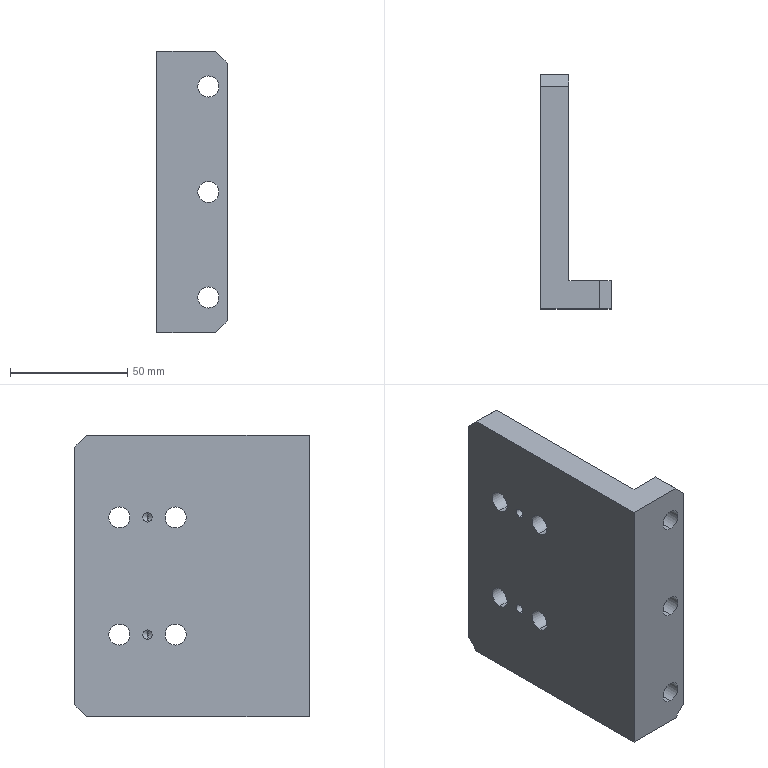Part | SolidWorks | features BaseBody 1 | 1 solid | 34 faces | box 30 x 100 x 120 mm | volume 163840 mm3 | cylinder 18 | plane 12 | cone 4 | commonest cylinder face diameters 9 x14 4 x4
STEP:
#1=CARTESIAN_POINT('',(5.,69.,-27.));
#2=VERTEX_POINT('',#1);
#3=CARTESIAN_POINT('',(5.,69.,-23.));
#4=VERTEX_POINT('',#3);
#5=CARTESIAN_POINT('',(5.,69.,-25.));
#6=DIRECTION('',(-1.,0.,0.));
#7=DIRECTION('',(0.,0.,1.));
#8=AXIS2_PLACEMENT_3D('',#5,#6,#7);
#9=CIRCLE('',#8,2.);
#10=EDGE_CURVE('',#2,#4,#9,.T.);
#11=ORIENTED_EDGE('',*,*,#10,.F.);
#12=CARTESIAN_POINT('',(0.,69.,-27.));
#13=VERTEX_POINT('',#12);
#14=CARTESIAN_POINT('',(0.,69.,-27.));
#15=DIRECTION('',(-1.,0.,0.));
#16=VECTOR('',#15,1000.);
#17=LINE('',#14,#16);
#18=EDGE_CURVE('',#2,#13,#17,.T.);
#19=ORIENTED_EDGE('',*,*,#18,.T.);
#20=CARTESIAN_POINT('',(0.,69.,-23.));
#21=VERTEX_POINT('',#20);
#22=CARTESIAN_POINT('',(0.,69.,-25.));
#23=DIRECTION('',(-1.,0.,0.));
#24=DIRECTION('',(0.,0.,1.));
#25=AXIS2_PLACEMENT_3D('',#22,#23,#24);
#26=CIRCLE('',#25,2.);
#27=EDGE_CURVE('',#13,#21,#26,.T.);
#28=ORIENTED_EDGE('',*,*,#27,.T.);
#29=CARTESIAN_POINT('',(0.,69.,-23.));
#30=DIRECTION('',(-1.,0.,0.));
#31=VECTOR('',#30,1000.);
#32=LINE('',#29,#31);
#33=EDGE_CURVE('',#4,#21,#32,.T.);
#34=ORIENTED_EDGE('',*,*,#33,.F.);
#35=EDGE_LOOP('',(#11,#19,#28,#34));
#36=FACE_OUTER_BOUND('',#35,.T.);
#37=CARTESIAN_POINT('',(0.,69.,-25.));
#38=DIRECTION('',(-1.,0.,0.));
#39=DIRECTION('',(0.,0.,1.));
#40=AXIS2_PLACEMENT_3D('',#37,#38,#39);
#41=CYLINDRICAL_SURFACE('',#40,2.);
#42=ADVANCED_FACE('',(#36),#41,.F.);
#43=CARTESIAN_POINT('',(6.202,69.,-25.));
#44=VERTEX_POINT('',#43);
#45=CARTESIAN_POINT('',(5.,69.,-23.));
#46=DIRECTION('',(-0.515,0.,0.8572));
#47=VECTOR('',#46,1000.);
#48=LINE('',#45,#47);
#49=EDGE_CURVE('',#44,#4,#48,.T.);
#50=ORIENTED_EDGE('',*,*,#49,.F.);
#51=CARTESIAN_POINT('',(5.,69.,-27.));
#52=DIRECTION('',(-0.515,0.,-0.8572));
#53=VECTOR('',#52,1000.);
#54=LINE('',#51,#53);
#55=EDGE_CURVE('',#44,#2,#54,.T.);
#56=ORIENTED_EDGE('',*,*,#55,.T.);
#57=ORIENTED_EDGE('',*,*,#10,.T.);
#58=EDGE_LOOP('',(#50,#56,#57));
#59=FACE_OUTER_BOUND('',#58,.T.);
#60=CARTESIAN_POINT('',(5.,69.,-25.));
#61=DIRECTION('',(-1.,0.,0.));
#62=DIRECTION('',(0.,0.,1.));
#63=AXIS2_PLACEMENT_3D('',#60,#61,#62);
#64=CONICAL_SURFACE('',#63,2.,1.03);
#65=ADVANCED_FACE('',(#59),#64,.F.);
#66=CARTESIAN_POINT('',(5.,69.,23.));
#67=VERTEX_POINT('',#66);
#68=CARTESIAN_POINT('',(5.,69.,27.));
#69=VERTEX_POINT('',#68);
#70=CARTESIAN_POINT('',(5.,69.,25.));
#71=DIRECTION('',(-1.,0.,0.));
#72=DIRECTION('',(0.,0.,1.));
#73=AXIS2_PLACEMENT_3D('',#70,#71,#72);
#74=CIRCLE('',#73,2.);
#75=EDGE_CURVE('',#67,#69,#74,.T.);
#76=ORIENTED_EDGE('',*,*,#75,.F.);
#77=CARTESIAN_POINT('',(0.,69.,23.));
#78=VERTEX_POINT('',#77);
#79=CARTESIAN_POINT('',(0.,69.,23.));
#80=DIRECTION('',(-1.,0.,0.));
#81=VECTOR('',#80,1000.);
#82=LINE('',#79,#81);
#83=EDGE_CURVE('',#67,#78,#82,.T.);
#84=ORIENTED_EDGE('',*,*,#83,.T.);
#85=CARTESIAN_POINT('',(0.,69.,27.));
#86=VERTEX_POINT('',#85);
#87=CARTESIAN_POINT('',(0.,69.,25.));
#88=DIRECTION('',(-1.,0.,0.));
#89=DIRECTION('',(0.,0.,1.));
#90=AXIS2_PLACEMENT_3D('',#87,#88,#89);
#91=CIRCLE('',#90,2.);
#92=EDGE_CURVE('',#78,#86,#91,.T.);
#93=ORIENTED_EDGE('',*,*,#92,.T.);
#94=CARTESIAN_POINT('',(0.,69.,27.));
#95=DIRECTION('',(-1.,0.,0.));
#96=VECTOR('',#95,1000.);
#97=LINE('',#94,#96);
#98=EDGE_CURVE('',#69,#86,#97,.T.);
#99=ORIENTED_EDGE('',*,*,#98,.F.);
#100=EDGE_LOOP('',(#76,#84,#93,#99));
#101=FACE_OUTER_BOUND('',#100,.T.);
#102=CARTESIAN_POINT('',(0.,69.,25.));
#103=DIRECTION('',(-1.,0.,0.));
#104=DIRECTION('',(0.,0.,1.));
#105=AXIS2_PLACEMENT_3D('',#102,#103,#104);
#106=CYLINDRICAL_SURFACE('',#105,2.);
#107=ADVANCED_FACE('',(#101),#106,.F.);
#108=CARTESIAN_POINT('',(6.202,69.,25.));
#109=VERTEX_POINT('',#108);
#110=CARTESIAN_POINT('',(5.,69.,27.));
#111=DIRECTION('',(-0.515,0.,0.8572));
#112=VECTOR('',#111,1000.);
#113=LINE('',#110,#112);
#114=EDGE_CURVE('',#109,#69,#113,.T.);
#115=ORIENTED_EDGE('',*,*,#114,.F.);
#116=CARTESIAN_POINT('',(5.,69.,23.));
#117=DIRECTION('',(-0.515,0.,-0.8572));
#118=VECTOR('',#117,1000.);
#119=LINE('',#116,#118);
#120=EDGE_CURVE('',#109,#67,#119,.T.);
#121=ORIENTED_EDGE('',*,*,#120,.T.);
#122=ORIENTED_EDGE('',*,*,#75,.T.);
#123=EDGE_LOOP('',(#115,#121,#122));
#124=FACE_OUTER_BOUND('',#123,.T.);
#125=CARTESIAN_POINT('',(5.,69.,25.));
#126=DIRECTION('',(-1.,0.,0.));
#127=DIRECTION('',(0.,0.,1.));
#128=AXIS2_PLACEMENT_3D('',#125,#126,#127);
#129=CONICAL_SURFACE('',#128,2.,1.03);
#130=ADVANCED_FACE('',(#124),#129,.F.);
#131=CARTESIAN_POINT('',(22.,0.,40.5));
#132=VERTEX_POINT('',#131);
#133=CARTESIAN_POINT('',(22.,0.,49.5));
#134=VERTEX_POINT('',#133);
#135=CARTESIAN_POINT('',(22.,0.,45.));
#136=DIRECTION('',(0.,1.,0.));
#137=DIRECTION('',(0.,0.,1.));
#138=AXIS2_PLACEMENT_3D('',#135,#136,#137);
#139=CIRCLE('',#138,4.5);
#140=EDGE_CURVE('',#132,#134,#139,.T.);
#141=ORIENTED_EDGE('',*,*,#140,.F.);
#142=CARTESIAN_POINT('',(22.,12.,40.5));
#143=VERTEX_POINT('',#142);
#144=CARTESIAN_POINT('',(22.,12.,40.5));
#145=DIRECTION('',(0.,1.,0.));
#146=VECTOR('',#145,1000.);
#147=LINE('',#144,#146);
#148=EDGE_CURVE('',#132,#143,#147,.T.);
#149=ORIENTED_EDGE('',*,*,#148,.T.);
#150=CARTESIAN_POINT('',(22.,12.,49.5));
#151=VERTEX_POINT('',#150);
#152=CARTESIAN_POINT('',(22.,12.,45.));
#153=DIRECTION('',(0.,1.,0.));
#154=DIRECTION('',(0.,0.,1.));
#155=AXIS2_PLACEMENT_3D('',#152,#153,#154);
#156=CIRCLE('',#155,4.5);
#157=EDGE_CURVE('',#143,#151,#156,.T.);
#158=ORIENTED_EDGE('',*,*,#157,.T.);
#159=CARTESIAN_POINT('',(22.,12.,49.5));
#160=DIRECTION('',(0.,1.,0.));
#161=VECTOR('',#160,1000.);
#162=LINE('',#159,#161);
#163=EDGE_CURVE('',#134,#151,#162,.T.);
#164=ORIENTED_EDGE('',*,*,#163,.F.);
#165=EDGE_LOOP('',(#141,#149,#158,#164));
#166=FACE_OUTER_BOUND('',#165,.T.);
#167=CARTESIAN_POINT('',(22.,12.,45.));
#168=DIRECTION('',(0.,1.,0.));
#169=DIRECTION('',(0.,0.,1.));
#170=AXIS2_PLACEMENT_3D('',#167,#168,#169);
#171=CYLINDRICAL_SURFACE('',#170,4.5);
#172=ADVANCED_FACE('',(#166),#171,.F.);
#173=CARTESIAN_POINT('',(22.,0.,-4.5));
#174=VERTEX_POINT('',#173);
#175=CARTESIAN_POINT('',(22.,0.,4.5));
#176=VERTEX_POINT('',#175);
#177=CARTESIAN_POINT('',(22.,0.,0.));
#178=DIRECTION('',(0.,1.,0.));
#179=DIRECTION('',(0.,0.,1.));
#180=AXIS2_PLACEMENT_3D('',#177,#178,#179);
#181=CIRCLE('',#180,4.5);
#182=EDGE_CURVE('',#174,#176,#181,.T.);
#183=ORIENTED_EDGE('',*,*,#182,.F.);
#184=CARTESIAN_POINT('',(22.,12.,-4.5));
#185=VERTEX_POINT('',#184);
#186=CARTESIAN_POINT('',(22.,12.,-4.5));
#187=DIRECTION('',(0.,1.,0.));
#188=VECTOR('',#187,1000.);
#189=LINE('',#186,#188);
#190=EDGE_CURVE('',#174,#185,#189,.T.);
#191=ORIENTED_EDGE('',*,*,#190,.T.);
#192=CARTESIAN_POINT('',(22.,12.,4.5));
#193=VERTEX_POINT('',#192);
#194=CARTESIAN_POINT('',(22.,12.,0.));
#195=DIRECTION('',(0.,1.,0.));
#196=DIRECTION('',(0.,0.,1.));
#197=AXIS2_PLACEMENT_3D('',#194,#195,#196);
#198=CIRCLE('',#197,4.5);
#199=EDGE_CURVE('',#185,#193,#198,.T.);
#200=ORIENTED_EDGE('',*,*,#199,.T.);
#201=CARTESIAN_POINT('',(22.,12.,4.5));
#202=DIRECTION('',(0.,1.,0.));
#203=VECTOR('',#202,1000.);
#204=LINE('',#201,#203);
#205=EDGE_CURVE('',#176,#193,#204,.T.);
#206=ORIENTED_EDGE('',*,*,#205,.F.);
#207=EDGE_LOOP('',(#183,#191,#200,#206));
#208=FACE_OUTER_BOUND('',#207,.T.);
#209=CARTESIAN_POINT('',(22.,12.,0.));
#210=DIRECTION('',(0.,1.,0.));
#211=DIRECTION('',(0.,0.,1.));
#212=AXIS2_PLACEMENT_3D('',#209,#210,#211);
#213=CYLINDRICAL_SURFACE('',#212,4.5);
#214=ADVANCED_FACE('',(#208),#213,.F.);
#215=CARTESIAN_POINT('',(22.,0.,-49.5));
#216=VERTEX_POINT('',#215);
#217=CARTESIAN_POINT('',(22.,0.,-40.5));
#218=VERTEX_POINT('',#217);
#219=CARTESIAN_POINT('',(22.,0.,-45.));
#220=DIRECTION('',(0.,1.,0.));
#221=DIRECTION('',(0.,0.,1.));
#222=AXIS2_PLACEMENT_3D('',#219,#220,#221);
#223=CIRCLE('',#222,4.5);
#224=EDGE_CURVE('',#216,#218,#223,.T.);
#225=ORIENTED_EDGE('',*,*,#224,.F.);
#226=CARTESIAN_POINT('',(22.,12.,-49.5));
#227=VERTEX_POINT('',#226);
#228=CARTESIAN_POINT('',(22.,12.,-49.5));
#229=DIRECTION('',(0.,1.,0.));
#230=VECTOR('',#229,1000.);
#231=LINE('',#228,#230);
#232=EDGE_CURVE('',#216,#227,#231,.T.);
#233=ORIENTED_EDGE('',*,*,#232,.T.);
#234=CARTESIAN_POINT('',(22.,12.,-40.5));
#235=VERTEX_POINT('',#234);
#236=CARTESIAN_POINT('',(22.,12.,-45.));
#237=DIRECTION('',(0.,1.,0.));
#238=DIRECTION('',(0.,0.,1.));
#239=AXIS2_PLACEMENT_3D('',#236,#237,#238);
#240=CIRCLE('',#239,4.5);
#241=EDGE_CURVE('',#227,#235,#240,.T.);
#242=ORIENTED_EDGE('',*,*,#241,.T.);
#243=CARTESIAN_POINT('',(22.,12.,-40.5));
#244=DIRECTION('',(0.,1.,0.));
#245=VECTOR('',#244,1000.);
#246=LINE('',#243,#245);
#247=EDGE_CURVE('',#218,#235,#246,.T.);
#248=ORIENTED_EDGE('',*,*,#247,.F.);
#249=EDGE_LOOP('',(#225,#233,#242,#248));
#250=FACE_OUTER_BOUND('',#249,.T.);
#251=CARTESIAN_POINT('',(22.,12.,-45.));
#252=DIRECTION('',(0.,1.,0.));
#253=DIRECTION('',(0.,0.,1.));
#254=AXIS2_PLACEMENT_3D('',#251,#252,#253);
#255=CYLINDRICAL_SURFACE('',#254,4.5);
#256=ADVANCED_FACE('',(#250),#255,.F.);
#257=CARTESIAN_POINT('',(0.,81.,29.5));
#258=VERTEX_POINT('',#257);
#259=CARTESIAN_POINT('',(0.,81.,20.5));
#260=VERTEX_POINT('',#259);
#261=CARTESIAN_POINT('',(0.,81.,25.));
#262=DIRECTION('',(1.,0.,0.));
#263=DIRECTION('',(0.,0.,-1.));
#264=AXIS2_PLACEMENT_3D('',#261,#262,#263);
#265=CIRCLE('',#264,4.5);
#266=EDGE_CURVE('',#258,#260,#265,.T.);
#267=ORIENTED_EDGE('',*,*,#266,.F.);
#268=CARTESIAN_POINT('',(12.,81.,29.5));
#269=VERTEX_POINT('',#268);
#270=CARTESIAN_POINT('',(12.,81.,29.5));
#271=DIRECTION('',(1.,0.,0.));
#272=VECTOR('',#271,1000.);
#273=LINE('',#270,#272);
#274=EDGE_CURVE('',#258,#269,#273,.T.);
#275=ORIENTED_EDGE('',*,*,#274,.T.);
#276=CARTESIAN_POINT('',(12.,81.,20.5));
#277=VERTEX_POINT('',#276);
#278=CARTESIAN_POINT('',(12.,81.,25.));
#279=DIRECTION('',(1.,0.,0.));
#280=DIRECTION('',(0.,0.,-1.));
#281=AXIS2_PLACEMENT_3D('',#278,#279,#280);
#282=CIRCLE('',#281,4.5);
#283=EDGE_CURVE('',#269,#277,#282,.T.);
#284=ORIENTED_EDGE('',*,*,#283,.T.);
#285=CARTESIAN_POINT('',(12.,81.,20.5));
#286=DIRECTION('',(1.,0.,0.));
#287=VECTOR('',#286,1000.);
#288=LINE('',#285,#287);
#289=EDGE_CURVE('',#260,#277,#288,.T.);
#290=ORIENTED_EDGE('',*,*,#289,.F.);
#291=EDGE_LOOP('',(#267,#275,#284,#290));
#292=FACE_OUTER_BOUND('',#291,.T.);
#293=CARTESIAN_POINT('',(12.,81.,25.));
#294=DIRECTION('',(1.,0.,0.));
#295=DIRECTION('',(0.,0.,-1.));
#296=AXIS2_PLACEMENT_3D('',#293,#294,#295);
#297=CYLINDRICAL_SURFACE('',#296,4.5);
#298=ADVANCED_FACE('',(#292),#297,.F.);
#299=CARTESIAN_POINT('',(0.,57.,-20.5));
#300=VERTEX_POINT('',#299);
#301=CARTESIAN_POINT('',(0.,57.,-29.5));
#302=VERTEX_POINT('',#301);
#303=CARTESIAN_POINT('',(0.,57.,-25.));
#304=DIRECTION('',(1.,0.,0.));
#305=DIRECTION('',(0.,0.,-1.));
#306=AXIS2_PLACEMENT_3D('',#303,#304,#305);
#307=CIRCLE('',#306,4.5);
#308=EDGE_CURVE('',#300,#302,#307,.T.);
#309=ORIENTED_EDGE('',*,*,#308,.F.);
#310=CARTESIAN_POINT('',(12.,57.,-20.5));
#311=VERTEX_POINT('',#310);
#312=CARTESIAN_POINT('',(12.,57.,-20.5));
#313=DIRECTION('',(1.,0.,0.));
#314=VECTOR('',#313,1000.);
#315=LINE('',#312,#314);
#316=EDGE_CURVE('',#300,#311,#315,.T.);
#317=ORIENTED_EDGE('',*,*,#316,.T.);
#318=CARTESIAN_POINT('',(12.,57.,-29.5));
#319=VERTEX_POINT('',#318);
#320=CARTESIAN_POINT('',(12.,57.,-25.));
#321=DIRECTION('',(1.,0.,0.));
#322=DIRECTION('',(0.,0.,-1.));
#323=AXIS2_PLACEMENT_3D('',#320,#321,#322);
#324=CIRCLE('',#323,4.5);
#325=EDGE_CURVE('',#311,#319,#324,.T.);
#326=ORIENTED_EDGE('',*,*,#325,.T.);
#327=CARTESIAN_POINT('',(12.,57.,-29.5));
#328=DIRECTION('',(1.,0.,0.));
#329=VECTOR('',#328,1000.);
#330=LINE('',#327,#329);
#331=EDGE_CURVE('',#302,#319,#330,.T.);
#332=ORIENTED_EDGE('',*,*,#331,.F.);
#333=EDGE_LOOP('',(#309,#317,#326,#332));
#334=FACE_OUTER_BOUND('',#333,.T.);
#335=CARTESIAN_POINT('',(12.,57.,-25.));
#336=DIRECTION('',(1.,0.,0.));
#337=DIRECTION('',(0.,0.,-1.));
#338=AXIS2_PLACEMENT_3D('',#335,#336,#337);
#339=CYLINDRICAL_SURFACE('',#338,4.5);
#340=ADVANCED_FACE('',(#334),#339,.F.);
#341=CARTESIAN_POINT('',(0.,57.,29.5));
#342=VERTEX_POINT('',#341);
#343=CARTESIAN_POINT('',(0.,57.,20.5));
#344=VERTEX_POINT('',#343);
#345=CARTESIAN_POINT('',(0.,57.,25.));
#346=DIRECTION('',(1.,0.,0.));
#347=DIRECTION('',(0.,0.,-1.));
#348=AXIS2_PLACEMENT_3D('',#345,#346,#347);
#349=CIRCLE('',#348,4.5);
#350=EDGE_CURVE('',#342,#344,#349,.T.);
#351=ORIENTED_EDGE('',*,*,#350,.F.);
#352=CARTESIAN_POINT('',(12.,57.,29.5));
#353=VERTEX_POINT('',#352);
#354=CARTESIAN_POINT('',(12.,57.,29.5));
#355=DIRECTION('',(1.,0.,0.));
#356=VECTOR('',#355,1000.);
#357=LINE('',#354,#356);
#358=EDGE_CURVE('',#342,#353,#357,.T.);
#359=ORIENTED_EDGE('',*,*,#358,.T.);
#360=CARTESIAN_POINT('',(12.,57.,20.5));
#361=VERTEX_POINT('',#360);
#362=CARTESIAN_POINT('',(12.,57.,25.));
#363=DIRECTION('',(1.,0.,0.));
#364=DIRECTION('',(0.,0.,-1.));
#365=AXIS2_PLACEMENT_3D('',#362,#363,#364);
#366=CIRCLE('',#365,4.5);
#367=EDGE_CURVE('',#353,#361,#366,.T.);
#368=ORIENTED_EDGE('',*,*,#367,.T.);
#369=CARTESIAN_POINT('',(12.,57.,20.5));
#370=DIRECTION('',(1.,0.,0.));
#371=VECTOR('',#370,1000.);
#372=LINE('',#369,#371);
#373=EDGE_CURVE('',#344,#361,#372,.T.);
#374=ORIENTED_EDGE('',*,*,#373,.F.);
#375=EDGE_LOOP('',(#351,#359,#368,#374));
#376=FACE_OUTER_BOUND('',#375,.T.);
#377=CARTESIAN_POINT('',(12.,57.,25.));
#378=DIRECTION('',(1.,0.,0.));
#379=DIRECTION('',(0.,0.,-1.));
#380=AXIS2_PLACEMENT_3D('',#377,#378,#379);
#381=CYLINDRICAL_SURFACE('',#380,4.5);
#382=ADVANCED_FACE('',(#376),#381,.F.);
#383=CARTESIAN_POINT('',(0.,81.,-20.5));
#384=VERTEX_POINT('',#383);
#385=CARTESIAN_POINT('',(0.,81.,-29.5));
#386=VERTEX_POINT('',#385);
#387=CARTESIAN_POINT('',(0.,81.,-25.));
#388=DIRECTION('',(1.,0.,0.));
#389=DIRECTION('',(0.,0.,-1.));
#390=AXIS2_PLACEMENT_3D('',#387,#388,#389);
#391=CIRCLE('',#390,4.5);
#392=EDGE_CURVE('',#384,#386,#391,.T.);
#393=ORIENTED_EDGE('',*,*,#392,.F.);
#394=CARTESIAN_POINT('',(12.,81.,-20.5));
#395=VERTEX_POINT('',#394);
#396=CARTESIAN_POINT('',(12.,81.,-20.5));
#397=DIRECTION('',(1.,0.,0.));
#398=VECTOR('',#397,1000.);
#399=LINE('',#396,#398);
#400=EDGE_CURVE('',#384,#395,#399,.T.);
#401=ORIENTED_EDGE('',*,*,#400,.T.);
#402=CARTESIAN_POINT('',(12.,81.,-29.5));
#403=VERTEX_POINT('',#402);
#404=CARTESIAN_POINT('',(12.,81.,-25.));
#405=DIRECTION('',(1.,0.,0.));
#406=DIRECTION('',(0.,0.,-1.));
#407=AXIS2_PLACEMENT_3D('',#404,#405,#406);
#408=CIRCLE('',#407,4.5);
#409=EDGE_CURVE('',#395,#403,#408,.T.);
#410=ORIENTED_EDGE('',*,*,#409,.T.);
#411=CARTESIAN_POINT('',(12.,81.,-29.5));
#412=DIRECTION('',(1.,0.,0.));
#413=VECTOR('',#412,1000.);
#414=LINE('',#411,#413);
#415=EDGE_CURVE('',#386,#403,#414,.T.);
#416=ORIENTED_EDGE('',*,*,#415,.F.);
#417=EDGE_LOOP('',(#393,#401,#410,#416));
#418=FACE_OUTER_BOUND('',#417,.T.);
#419=CARTESIAN_POINT('',(12.,81.,-25.));
#420=DIRECTION('',(1.,0.,0.));
#421=DIRECTION('',(0.,0.,-1.));
#422=AXIS2_PLACEMENT_3D('',#419,#420,#421);
#423=CYLINDRICAL_SURFACE('',#422,4.5);
#424=ADVANCED_FACE('',(#418),#423,.F.);
#425=CARTESIAN_POINT('',(0.,95.,60.));
#426=VERTEX_POINT('',#425);
#427=CARTESIAN_POINT('',(0.,100.,55.));
#428=VERTEX_POINT('',#427);
#429=CARTESIAN_POINT('',(0.,100.,55.));
#430=DIRECTION('',(0.,0.7071,-0.7071));
#431=VECTOR('',#430,1000.);
#432=LINE('',#429,#431);
#433=EDGE_CURVE('',#426,#428,#432,.T.);
#434=ORIENTED_EDGE('',*,*,#433,.F.);
#435=CARTESIAN_POINT('',(12.,95.,60.));
#436=VERTEX_POINT('',#435);
#437=CARTESIAN_POINT('',(0.,95.,60.));
#438=DIRECTION('',(-1.,0.,0.));
#439=VECTOR('',#438,1000.);
#440=LINE('',#437,#439);
#441=EDGE_CURVE('',#436,#426,#440,.T.);
#442=ORIENTED_EDGE('',*,*,#441,.F.);
#443=CARTESIAN_POINT('',(12.,100.,55.));
#444=VERTEX_POINT('',#443);
#445=CARTESIAN_POINT('',(12.,97.5,57.5));
#446=DIRECTION('',(0.,-0.7071,0.7071));
#447=VECTOR('',#446,1000.);
#448=LINE('',#445,#447);
#449=EDGE_CURVE('',#444,#436,#448,.T.);
#450=ORIENTED_EDGE('',*,*,#449,.F.);
#451=CARTESIAN_POINT('',(12.,100.,55.));
#452=DIRECTION('',(1.,0.,0.));
#453=VECTOR('',#452,1000.);
#454=LINE('',#451,#453);
#455=EDGE_CURVE('',#428,#444,#454,.T.);
#456=ORIENTED_EDGE('',*,*,#455,.F.);
#457=EDGE_LOOP('',(#434,#442,#450,#456));
#458=FACE_OUTER_BOUND('',#457,.T.);
#459=CARTESIAN_POINT('',(0.,100.,55.));
#460=DIRECTION('',(0.,0.7071,0.7071));
#461=DIRECTION('',(1.,0.,0.));
#462=AXIS2_PLACEMENT_3D('',#459,#460,#461);
#463=PLANE('',#462);
#464=ADVANCED_FACE('',(#458),#463,.T.);
#465=CARTESIAN_POINT('',(0.,100.,-55.));
#466=VERTEX_POINT('',#465);
#467=CARTESIAN_POINT('',(0.,95.,-60.));
#468=VERTEX_POINT('',#467);
#469=CARTESIAN_POINT('',(0.,95.,-60.));
#470=DIRECTION('',(0.,-0.7071,-0.7071));
#471=VECTOR('',#470,1000.);
#472=LINE('',#469,#471);
#473=EDGE_CURVE('',#466,#468,#472,.T.);
#474=ORIENTED_EDGE('',*,*,#473,.F.);
#475=CARTESIAN_POINT('',(12.,100.,-55.));
#476=VERTEX_POINT('',#475);
#477=CARTESIAN_POINT('',(0.,100.,-55.));
#478=DIRECTION('',(-1.,0.,0.));
#479=VECTOR('',#478,1000.);
#480=LINE('',#477,#479);
#481=EDGE_CURVE('',#476,#466,#480,.T.);
#482=ORIENTED_EDGE('',*,*,#481,.F.);
#483=CARTESIAN_POINT('',(12.,95.,-60.));
#484=VERTEX_POINT('',#483);
#485=CARTESIAN_POINT('',(12.,157.5,2.5));
#486=DIRECTION('',(0.,0.7071,0.7071));
#487=VECTOR('',#486,1000.);
#488=LINE('',#485,#487);
#489=EDGE_CURVE('',#484,#476,#488,.T.);
#490=ORIENTED_EDGE('',*,*,#489,.F.);
#491=CARTESIAN_POINT('',(0.,95.,-60.));
#492=DIRECTION('',(1.,0.,0.));
#493=VECTOR('',#492,1000.);
#494=LINE('',#491,#493);
#495=EDGE_CURVE('',#468,#484,#494,.T.);
#496=ORIENTED_EDGE('',*,*,#495,.F.);
#497=EDGE_LOOP('',(#474,#482,#490,#496));
#498=FACE_OUTER_BOUND('',#497,.T.);
#499=CARTESIAN_POINT('',(0.,95.,-60.));
#500=DIRECTION('',(0.,-0.7071,0.7071));
#501=DIRECTION('',(-1.,0.,0.));
#502=AXIS2_PLACEMENT_3D('',#499,#500,#501);
#503=PLANE('',#502);
#504=ADVANCED_FACE('',(#498),#503,.F.);
#505=CARTESIAN_POINT('',(30.,12.,-55.));
#506=VERTEX_POINT('',#505);
#507=CARTESIAN_POINT('',(25.,12.,-60.));
#508=VERTEX_POINT('',#507);
#509=CARTESIAN_POINT('',(72.5,12.,-12.5));
#510=DIRECTION('',(-0.7071,0.,-0.7071));
#511=VECTOR('',#510,1000.);
#512=LINE('',#509,#511);
#513=EDGE_CURVE('',#506,#508,#512,.T.);
#514=ORIENTED_EDGE('',*,*,#513,.F.);
#515=CARTESIAN_POINT('',(30.,0.,-55.));
#516=VERTEX_POINT('',#515);
#517=CARTESIAN_POINT('',(30.,12.,-55.));
#518=DIRECTION('',(0.,1.,0.));
#519=VECTOR('',#518,1000.);
#520=LINE('',#517,#519);
#521=EDGE_CURVE('',#516,#506,#520,.T.);
#522=ORIENTED_EDGE('',*,*,#521,.F.);
#523=CARTESIAN_POINT('',(25.,0.,-60.));
#524=VERTEX_POINT('',#523);
#525=CARTESIAN_POINT('',(25.,0.,-60.));
#526=DIRECTION('',(0.7071,0.,0.7071));
#527=VECTOR('',#526,1000.);
#528=LINE('',#525,#527);
#529=EDGE_CURVE('',#524,#516,#528,.T.);
#530=ORIENTED_EDGE('',*,*,#529,.F.);
#531=CARTESIAN_POINT('',(25.,0.,-60.));
#532=DIRECTION('',(0.,-1.,0.));
#533=VECTOR('',#532,1000.);
#534=LINE('',#531,#533);
#535=EDGE_CURVE('',#508,#524,#534,.T.);
#536=ORIENTED_EDGE('',*,*,#535,.F.);
#537=EDGE_LOOP('',(#514,#522,#530,#536));
#538=FACE_OUTER_BOUND('',#537,.T.);
#539=CARTESIAN_POINT('',(25.,0.,-60.));
#540=DIRECTION('',(-0.7071,0.,0.7071));
#541=DIRECTION('',(0.,1.,0.));
#542=AXIS2_PLACEMENT_3D('',#539,#540,#541);
#543=PLANE('',#542);
#544=ADVANCED_FACE('',(#538),#543,.F.);
#545=CARTESIAN_POINT('',(25.,12.,60.));
#546=VERTEX_POINT('',#545);
#547=CARTESIAN_POINT('',(30.,12.,55.));
#548=VERTEX_POINT('',#547);
#549=CARTESIAN_POINT('',(12.5,12.,72.5));
#550=DIRECTION('',(0.7071,0.,-0.7071));
#551=VECTOR('',#550,1000.);
#552=LINE('',#549,#551);
#553=EDGE_CURVE('',#546,#548,#552,.T.);
#554=ORIENTED_EDGE('',*,*,#553,.F.);
#555=CARTESIAN_POINT('',(25.,0.,60.));
#556=VERTEX_POINT('',#555);
#557=CARTESIAN_POINT('',(25.,12.,60.));
#558=DIRECTION('',(0.,1.,0.));
#559=VECTOR('',#558,1000.);
#560=LINE('',#557,#559);
#561=EDGE_CURVE('',#556,#546,#560,.T.);
#562=ORIENTED_EDGE('',*,*,#561,.F.);
#563=CARTESIAN_POINT('',(30.,0.,55.));
#564=VERTEX_POINT('',#563);
#565=CARTESIAN_POINT('',(30.,0.,55.));
#566=DIRECTION('',(-0.7071,0.,0.7071));
#567=VECTOR('',#566,1000.);
#568=LINE('',#565,#567);
#569=EDGE_CURVE('',#564,#556,#568,.T.);
#570=ORIENTED_EDGE('',*,*,#569,.F.);
#571=CARTESIAN_POINT('',(30.,0.,55.));
#572=DIRECTION('',(0.,-1.,0.));
#573=VECTOR('',#572,1000.);
#574=LINE('',#571,#573);
#575=EDGE_CURVE('',#548,#564,#574,.T.);
#576=ORIENTED_EDGE('',*,*,#575,.F.);
#577=EDGE_LOOP('',(#554,#562,#570,#576));
#578=FACE_OUTER_BOUND('',#577,.T.);
#579=CARTESIAN_POINT('',(30.,12.,55.));
#580=DIRECTION('',(0.7071,0.,0.7071));
#581=DIRECTION('',(0.,-1.,0.));
#582=AXIS2_PLACEMENT_3D('',#579,#580,#581);
#583=PLANE('',#582);
#584=ADVANCED_FACE('',(#578),#583,.T.);
#585=CARTESIAN_POINT('',(12.,12.,-60.));
#586=VERTEX_POINT('',#585);
#587=CARTESIAN_POINT('',(0.,12.,-60.));
#588=DIRECTION('',(1.,0.,0.));
#589=VECTOR('',#588,1000.);
#590=LINE('',#587,#589);
#591=EDGE_CURVE('',#586,#508,#590,.T.);
#592=ORIENTED_EDGE('',*,*,#591,.T.);
#593=ORIENTED_EDGE('',*,*,#535,.T.);
#594=CARTESIAN_POINT('',(0.,0.,-60.));
#595=VERTEX_POINT('',#594);
#596=CARTESIAN_POINT('',(0.,0.,-60.));
#597=DIRECTION('',(1.,0.,0.));
#598=VECTOR('',#597,1000.);
#599=LINE('',#596,#598);
#600=EDGE_CURVE('',#595,#524,#599,.T.);
#601=ORIENTED_EDGE('',*,*,#600,.F.);
#602=CARTESIAN_POINT('',(0.,100.,-60.));
#603=DIRECTION('',(0.,-1.,0.));
#604=VECTOR('',#603,1000.);
#605=LINE('',#602,#604);
#606=EDGE_CURVE('',#468,#595,#605,.T.);
#607=ORIENTED_EDGE('',*,*,#606,.F.);
#608=ORIENTED_EDGE('',*,*,#495,.T.);
#609=CARTESIAN_POINT('',(12.,100.,-60.));
#610=DIRECTION('',(0.,-1.,0.));
#611=VECTOR('',#610,1000.);
#612=LINE('',#609,#611);
#613=EDGE_CURVE('',#484,#586,#612,.T.);
#614=ORIENTED_EDGE('',*,*,#613,.T.);
#615=EDGE_LOOP('',(#592,#593,#601,#607,#608,#614));
#616=FACE_OUTER_BOUND('',#615,.T.);
#617=CARTESIAN_POINT('',(0.,0.,-60.));
#618=DIRECTION('',(0.,0.,-1.));
#619=DIRECTION('',(0.,-1.,0.));
#620=AXIS2_PLACEMENT_3D('',#617,#618,#619);
#621=PLANE('',#620);
#622=ADVANCED_FACE('',(#616),#621,.T.);
#623=CARTESIAN_POINT('',(0.,0.,60.));
#624=VERTEX_POINT('',#623);
#625=CARTESIAN_POINT('',(0.,0.,60.));
#626=DIRECTION('',(1.,0.,0.));
#627=VECTOR('',#626,1000.);
#628=LINE('',#625,#627);
#629=EDGE_CURVE('',#624,#556,#628,.T.);
#630=ORIENTED_EDGE('',*,*,#629,.T.);
#631=ORIENTED_EDGE('',*,*,#561,.T.);
#632=CARTESIAN_POINT('',(12.,12.,60.));
#633=VERTEX_POINT('',#632);
#634=CARTESIAN_POINT('',(0.,12.,60.));
#635=DIRECTION('',(1.,0.,0.));
#636=VECTOR('',#635,1000.);
#637=LINE('',#634,#636);
#638=EDGE_CURVE('',#633,#546,#637,.T.);
#639=ORIENTED_EDGE('',*,*,#638,.F.);
#640=CARTESIAN_POINT('',(12.,100.,60.));
#641=DIRECTION('',(0.,-1.,0.));
#642=VECTOR('',#641,1000.);
#643=LINE('',#640,#642);
#644=EDGE_CURVE('',#436,#633,#643,.T.);
#645=ORIENTED_EDGE('',*,*,#644,.F.);
#646=ORIENTED_EDGE('',*,*,#441,.T.);
#647=CARTESIAN_POINT('',(0.,100.,60.));
#648=DIRECTION('',(0.,-1.,0.));
#649=VECTOR('',#648,1000.);
#650=LINE('',#647,#649);
#651=EDGE_CURVE('',#426,#624,#650,.T.);
#652=ORIENTED_EDGE('',*,*,#651,.T.);
#653=EDGE_LOOP('',(#630,#631,#639,#645,#646,#652));
#654=FACE_OUTER_BOUND('',#653,.T.);
#655=CARTESIAN_POINT('',(0.,0.,60.));
#656=DIRECTION('',(0.,0.,-1.));
#657=DIRECTION('',(0.,-1.,0.));
#658=AXIS2_PLACEMENT_3D('',#655,#656,#657);
#659=PLANE('',#658);
#660=ADVANCED_FACE('',(#654),#659,.F.);
#661=CARTESIAN_POINT('',(0.,81.,-25.));
#662=DIRECTION('',(1.,0.,0.));
#663=DIRECTION('',(0.,0.,-1.));
#664=AXIS2_PLACEMENT_3D('',#661,#662,#663);
#665=CIRCLE('',#664,4.5);
#666=EDGE_CURVE('',#386,#384,#665,.T.);
#667=ORIENTED_EDGE('',*,*,#666,.T.);
#668=ORIENTED_EDGE('',*,*,#392,.T.);
#669=EDGE_LOOP('',(#667,#668));
#670=FACE_BOUND('',#669,.T.);
#671=CARTESIAN_POINT('',(0.,57.,25.));
#672=DIRECTION('',(1.,0.,0.));
#673=DIRECTION('',(0.,0.,-1.));
#674=AXIS2_PLACEMENT_3D('',#671,#672,#673);
#675=CIRCLE('',#674,4.5);
#676=EDGE_CURVE('',#344,#342,#675,.T.);
#677=ORIENTED_EDGE('',*,*,#676,.T.);
#678=ORIENTED_EDGE('',*,*,#350,.T.);
#679=EDGE_LOOP('',(#677,#678));
#680=FACE_BOUND('',#679,.T.);
#681=CARTESIAN_POINT('',(0.,57.,-25.));
#682=DIRECTION('',(1.,0.,0.));
#683=DIRECTION('',(0.,0.,-1.));
#684=AXIS2_PLACEMENT_3D('',#681,#682,#683);
#685=CIRCLE('',#684,4.5);
#686=EDGE_CURVE('',#302,#300,#685,.T.);
#687=ORIENTED_EDGE('',*,*,#686,.T.);
#688=ORIENTED_EDGE('',*,*,#308,.T.);
#689=EDGE_LOOP('',(#687,#688));
#690=FACE_BOUND('',#689,.T.);
#691=CARTESIAN_POINT('',(0.,81.,25.));
#692=DIRECTION('',(1.,0.,0.));
#693=DIRECTION('',(0.,0.,-1.));
#694=AXIS2_PLACEMENT_3D('',#691,#692,#693);
#695=CIRCLE('',#694,4.5);
#696=EDGE_CURVE('',#260,#258,#695,.T.);
#697=ORIENTED_EDGE('',*,*,#696,.T.);
#698=ORIENTED_EDGE('',*,*,#266,.T.);
#699=EDGE_LOOP('',(#697,#698));
#700=FACE_BOUND('',#699,.T.);
#701=CARTESIAN_POINT('',(0.,69.,25.));
#702=DIRECTION('',(-1.,0.,0.));
#703=DIRECTION('',(0.,0.,1.));
#704=AXIS2_PLACEMENT_3D('',#701,#702,#703);
#705=CIRCLE('',#704,2.);
#706=EDGE_CURVE('',#86,#78,#705,.T.);
#707=ORIENTED_EDGE('',*,*,#706,.F.);
#708=ORIENTED_EDGE('',*,*,#92,.F.);
#709=EDGE_LOOP('',(#707,#708));
#710=FACE_BOUND('',#709,.T.);
#711=CARTESIAN_POINT('',(0.,69.,-25.));
#712=DIRECTION('',(-1.,0.,0.));
#713=DIRECTION('',(0.,0.,1.));
#714=AXIS2_PLACEMENT_3D('',#711,#712,#713);
#715=CIRCLE('',#714,2.);
#716=EDGE_CURVE('',#21,#13,#715,.T.);
#717=ORIENTED_EDGE('',*,*,#716,.F.);
#718=ORIENTED_EDGE('',*,*,#27,.F.);
#719=EDGE_LOOP('',(#717,#718));
#720=FACE_BOUND('',#719,.T.);
#721=CARTESIAN_POINT('',(0.,100.,60.));
#722=DIRECTION('',(0.,0.,-1.));
#723=VECTOR('',#722,1000.);
#724=LINE('',#721,#723);
#725=EDGE_CURVE('',#428,#466,#724,.T.);
#726=ORIENTED_EDGE('',*,*,#725,.T.);
#727=ORIENTED_EDGE('',*,*,#473,.T.);
#728=ORIENTED_EDGE('',*,*,#606,.T.);
#729=CARTESIAN_POINT('',(0.,0.,60.));
#730=DIRECTION('',(0.,0.,-1.));
#731=VECTOR('',#730,1000.);
#732=LINE('',#729,#731);
#733=EDGE_CURVE('',#624,#595,#732,.T.);
#734=ORIENTED_EDGE('',*,*,#733,.F.);
#735=ORIENTED_EDGE('',*,*,#651,.F.);
#736=ORIENTED_EDGE('',*,*,#433,.T.);
#737=EDGE_LOOP('',(#726,#727,#728,#734,#735,#736));
#738=FACE_OUTER_BOUND('',#737,.T.);
#739=CARTESIAN_POINT('',(0.,100.,60.));
#740=DIRECTION('',(1.,0.,0.));
#741=DIRECTION('',(0.,1.,0.));
#742=AXIS2_PLACEMENT_3D('',#739,#740,#741);
#743=PLANE('',#742);
#744=ADVANCED_FACE('',(#670,#680,#690,#700,#710,#720,#738),#743,.F.);
#745=CARTESIAN_POINT('',(12.,100.,60.));
#746=DIRECTION('',(0.,0.,-1.));
#747=VECTOR('',#746,1000.);
#748=LINE('',#745,#747);
#749=EDGE_CURVE('',#444,#476,#748,.T.);
#750=ORIENTED_EDGE('',*,*,#749,.T.);
#751=ORIENTED_EDGE('',*,*,#481,.T.);
#752=ORIENTED_EDGE('',*,*,#725,.F.);
#753=ORIENTED_EDGE('',*,*,#455,.T.);
#754=EDGE_LOOP('',(#750,#751,#752,#753));
#755=FACE_OUTER_BOUND('',#754,.T.);
#756=CARTESIAN_POINT('',(0.,100.,60.));
#757=DIRECTION('',(0.,1.,0.));
#758=DIRECTION('',(1.,0.,0.));
#759=AXIS2_PLACEMENT_3D('',#756,#757,#758);
#760=PLANE('',#759);
#761=ADVANCED_FACE('',(#755),#760,.T.);
#762=CARTESIAN_POINT('',(12.,81.,-25.));
#763=DIRECTION('',(1.,0.,0.));
#764=DIRECTION('',(0.,0.,-1.));
#765=AXIS2_PLACEMENT_3D('',#762,#763,#764);
#766=CIRCLE('',#765,4.5);
#767=EDGE_CURVE('',#403,#395,#766,.T.);
#768=ORIENTED_EDGE('',*,*,#767,.F.);
#769=ORIENTED_EDGE('',*,*,#409,.F.);
#770=EDGE_LOOP('',(#768,#769));
#771=FACE_BOUND('',#770,.T.);
#772=CARTESIAN_POINT('',(12.,57.,25.));
#773=DIRECTION('',(1.,0.,0.));
#774=DIRECTION('',(0.,0.,-1.));
#775=AXIS2_PLACEMENT_3D('',#772,#773,#774);
#776=CIRCLE('',#775,4.5);
#777=EDGE_CURVE('',#361,#353,#776,.T.);
#778=ORIENTED_EDGE('',*,*,#777,.F.);
#779=ORIENTED_EDGE('',*,*,#367,.F.);
#780=EDGE_LOOP('',(#778,#779));
#781=FACE_BOUND('',#780,.T.);
#782=CARTESIAN_POINT('',(12.,57.,-25.));
#783=DIRECTION('',(1.,0.,0.));
#784=DIRECTION('',(0.,0.,-1.));
#785=AXIS2_PLACEMENT_3D('',#782,#783,#784);
#786=CIRCLE('',#785,4.5);
#787=EDGE_CURVE('',#319,#311,#786,.T.);
#788=ORIENTED_EDGE('',*,*,#787,.F.);
#789=ORIENTED_EDGE('',*,*,#325,.F.);
#790=EDGE_LOOP('',(#788,#789));
#791=FACE_BOUND('',#790,.T.);
#792=CARTESIAN_POINT('',(12.,81.,25.));
#793=DIRECTION('',(1.,0.,0.));
#794=DIRECTION('',(0.,0.,-1.));
#795=AXIS2_PLACEMENT_3D('',#792,#793,#794);
#796=CIRCLE('',#795,4.5);
#797=EDGE_CURVE('',#277,#269,#796,.T.);
#798=ORIENTED_EDGE('',*,*,#797,.F.);
#799=ORIENTED_EDGE('',*,*,#283,.F.);
#800=EDGE_LOOP('',(#798,#799));
#801=FACE_BOUND('',#800,.T.);
#802=ORIENTED_EDGE('',*,*,#613,.F.);
#803=ORIENTED_EDGE('',*,*,#489,.T.);
#804=ORIENTED_EDGE('',*,*,#749,.F.);
#805=ORIENTED_EDGE('',*,*,#449,.T.);
#806=ORIENTED_EDGE('',*,*,#644,.T.);
#807=CARTESIAN_POINT('',(12.,12.,60.));
#808=DIRECTION('',(0.,0.,-1.));
#809=VECTOR('',#808,1000.);
#810=LINE('',#807,#809);
#811=EDGE_CURVE('',#633,#586,#810,.T.);
#812=ORIENTED_EDGE('',*,*,#811,.T.);
#813=EDGE_LOOP('',(#802,#803,#804,#805,#806,#812));
#814=FACE_OUTER_BOUND('',#813,.T.);
#815=CARTESIAN_POINT('',(12.,100.,60.));
#816=DIRECTION('',(1.,0.,0.));
#817=DIRECTION('',(0.,1.,0.));
#818=AXIS2_PLACEMENT_3D('',#815,#816,#817);
#819=PLANE('',#818);
#820=ADVANCED_FACE('',(#771,#781,#791,#801,#814),#819,.T.);
#821=CARTESIAN_POINT('',(22.,12.,-45.));
#822=DIRECTION('',(0.,1.,0.));
#823=DIRECTION('',(0.,0.,1.));
#824=AXIS2_PLACEMENT_3D('',#821,#822,#823);
#825=CIRCLE('',#824,4.5);
#826=EDGE_CURVE('',#235,#227,#825,.T.);
#827=ORIENTED_EDGE('',*,*,#826,.F.);
#828=ORIENTED_EDGE('',*,*,#241,.F.);
#829=EDGE_LOOP('',(#827,#828));
#830=FACE_BOUND('',#829,.T.);
#831=CARTESIAN_POINT('',(22.,12.,0.));
#832=DIRECTION('',(0.,1.,0.));
#833=DIRECTION('',(0.,0.,1.));
#834=AXIS2_PLACEMENT_3D('',#831,#832,#833);
#835=CIRCLE('',#834,4.5);
#836=EDGE_CURVE('',#193,#185,#835,.T.);
#837=ORIENTED_EDGE('',*,*,#836,.F.);
#838=ORIENTED_EDGE('',*,*,#199,.F.);
#839=EDGE_LOOP('',(#837,#838));
#840=FACE_BOUND('',#839,.T.);
#841=CARTESIAN_POINT('',(22.,12.,45.));
#842=DIRECTION('',(0.,1.,0.));
#843=DIRECTION('',(0.,0.,1.));
#844=AXIS2_PLACEMENT_3D('',#841,#842,#843);
#845=CIRCLE('',#844,4.5);
#846=EDGE_CURVE('',#151,#143,#845,.T.);
#847=ORIENTED_EDGE('',*,*,#846,.F.);
#848=ORIENTED_EDGE('',*,*,#157,.F.);
#849=EDGE_LOOP('',(#847,#848));
#850=FACE_BOUND('',#849,.T.);
#851=ORIENTED_EDGE('',*,*,#638,.T.);
#852=ORIENTED_EDGE('',*,*,#553,.T.);
#853=CARTESIAN_POINT('',(30.,12.,60.));
#854=DIRECTION('',(0.,0.,-1.));
#855=VECTOR('',#854,1000.);
#856=LINE('',#853,#855);
#857=EDGE_CURVE('',#548,#506,#856,.T.);
#858=ORIENTED_EDGE('',*,*,#857,.T.);
#859=ORIENTED_EDGE('',*,*,#513,.T.);
#860=ORIENTED_EDGE('',*,*,#591,.F.);
#861=ORIENTED_EDGE('',*,*,#811,.F.);
#862=EDGE_LOOP('',(#851,#852,#858,#859,#860,#861));
#863=FACE_OUTER_BOUND('',#862,.T.);
#864=CARTESIAN_POINT('',(0.,12.,60.));
#865=DIRECTION('',(0.,1.,0.));
#866=DIRECTION('',(1.,0.,0.));
#867=AXIS2_PLACEMENT_3D('',#864,#865,#866);
#868=PLANE('',#867);
#869=ADVANCED_FACE('',(#830,#840,#850,#863),#868,.T.);
#870=ORIENTED_EDGE('',*,*,#857,.F.);
#871=ORIENTED_EDGE('',*,*,#575,.T.);
#872=CARTESIAN_POINT('',(30.,0.,60.));
#873=DIRECTION('',(0.,0.,-1.));
#874=VECTOR('',#873,1000.);
#875=LINE('',#872,#874);
#876=EDGE_CURVE('',#564,#516,#875,.T.);
#877=ORIENTED_EDGE('',*,*,#876,.T.);
#878=ORIENTED_EDGE('',*,*,#521,.T.);
#879=EDGE_LOOP('',(#870,#871,#877,#878));
#880=FACE_OUTER_BOUND('',#879,.T.);
#881=CARTESIAN_POINT('',(30.,12.,60.));
#882=DIRECTION('',(1.,0.,0.));
#883=DIRECTION('',(0.,1.,0.));
#884=AXIS2_PLACEMENT_3D('',#881,#882,#883);
#885=PLANE('',#884);
#886=ADVANCED_FACE('',(#880),#885,.T.);
#887=CARTESIAN_POINT('',(22.,0.,-45.));
#888=DIRECTION('',(0.,1.,0.));
#889=DIRECTION('',(0.,0.,1.));
#890=AXIS2_PLACEMENT_3D('',#887,#888,#889);
#891=CIRCLE('',#890,4.5);
#892=EDGE_CURVE('',#218,#216,#891,.T.);
#893=ORIENTED_EDGE('',*,*,#892,.T.);
#894=ORIENTED_EDGE('',*,*,#224,.T.);
#895=EDGE_LOOP('',(#893,#894));
#896=FACE_BOUND('',#895,.T.);
#897=CARTESIAN_POINT('',(22.,0.,0.));
#898=DIRECTION('',(0.,1.,0.));
#899=DIRECTION('',(0.,0.,1.));
#900=AXIS2_PLACEMENT_3D('',#897,#898,#899);
#901=CIRCLE('',#900,4.5);
#902=EDGE_CURVE('',#176,#174,#901,.T.);
#903=ORIENTED_EDGE('',*,*,#902,.T.);
#904=ORIENTED_EDGE('',*,*,#182,.T.);
#905=EDGE_LOOP('',(#903,#904));
#906=FACE_BOUND('',#905,.T.);
#907=CARTESIAN_POINT('',(22.,0.,45.));
#908=DIRECTION('',(0.,1.,0.));
#909=DIRECTION('',(0.,0.,1.));
#910=AXIS2_PLACEMENT_3D('',#907,#908,#909);
#911=CIRCLE('',#910,4.5);
#912=EDGE_CURVE('',#134,#132,#911,.T.);
#913=ORIENTED_EDGE('',*,*,#912,.T.);
#914=ORIENTED_EDGE('',*,*,#140,.T.);
#915=EDGE_LOOP('',(#913,#914));
#916=FACE_BOUND('',#915,.T.);
#917=ORIENTED_EDGE('',*,*,#876,.F.);
#918=ORIENTED_EDGE('',*,*,#569,.T.);
#919=ORIENTED_EDGE('',*,*,#629,.F.);
#920=ORIENTED_EDGE('',*,*,#733,.T.);
#921=ORIENTED_EDGE('',*,*,#600,.T.);
#922=ORIENTED_EDGE('',*,*,#529,.T.);
#923=EDGE_LOOP('',(#917,#918,#919,#920,#921,#922));
#924=FACE_OUTER_BOUND('',#923,.T.);
#925=CARTESIAN_POINT('',(0.,0.,60.));
#926=DIRECTION('',(0.,1.,0.));
#927=DIRECTION('',(1.,0.,0.));
#928=AXIS2_PLACEMENT_3D('',#925,#926,#927);
#929=PLANE('',#928);
#930=ADVANCED_FACE('',(#896,#906,#916,#924),#929,.F.);
#931=ORIENTED_EDGE('',*,*,#400,.F.);
#932=ORIENTED_EDGE('',*,*,#666,.F.);
#933=ORIENTED_EDGE('',*,*,#415,.T.);
#934=ORIENTED_EDGE('',*,*,#767,.T.);
#935=EDGE_LOOP('',(#931,#932,#933,#934));
#936=FACE_OUTER_BOUND('',#935,.T.);
#937=CARTESIAN_POINT('',(12.,81.,-25.));
#938=DIRECTION('',(1.,0.,0.));
#939=DIRECTION('',(0.,0.,-1.));
#940=AXIS2_PLACEMENT_3D('',#937,#938,#939);
#941=CYLINDRICAL_SURFACE('',#940,4.5);
#942=ADVANCED_FACE('',(#936),#941,.F.);
#943=ORIENTED_EDGE('',*,*,#358,.F.);
#944=ORIENTED_EDGE('',*,*,#676,.F.);
#945=ORIENTED_EDGE('',*,*,#373,.T.);
#946=ORIENTED_EDGE('',*,*,#777,.T.);
#947=EDGE_LOOP('',(#943,#944,#945,#946));
#948=FACE_OUTER_BOUND('',#947,.T.);
#949=CARTESIAN_POINT('',(12.,57.,25.));
#950=DIRECTION('',(1.,0.,0.));
#951=DIRECTION('',(0.,0.,-1.));
#952=AXIS2_PLACEMENT_3D('',#949,#950,#951);
#953=CYLINDRICAL_SURFACE('',#952,4.5);
#954=ADVANCED_FACE('',(#948),#953,.F.);
#955=ORIENTED_EDGE('',*,*,#316,.F.);
#956=ORIENTED_EDGE('',*,*,#686,.F.);
#957=ORIENTED_EDGE('',*,*,#331,.T.);
#958=ORIENTED_EDGE('',*,*,#787,.T.);
#959=EDGE_LOOP('',(#955,#956,#957,#958));
#960=FACE_OUTER_BOUND('',#959,.T.);
#961=CARTESIAN_POINT('',(12.,57.,-25.));
#962=DIRECTION('',(1.,0.,0.));
#963=DIRECTION('',(0.,0.,-1.));
#964=AXIS2_PLACEMENT_3D('',#961,#962,#963);
#965=CYLINDRICAL_SURFACE('',#964,4.5);
#966=ADVANCED_FACE('',(#960),#965,.F.);
#967=ORIENTED_EDGE('',*,*,#274,.F.);
#968=ORIENTED_EDGE('',*,*,#696,.F.);
#969=ORIENTED_EDGE('',*,*,#289,.T.);
#970=ORIENTED_EDGE('',*,*,#797,.T.);
#971=EDGE_LOOP('',(#967,#968,#969,#970));
#972=FACE_OUTER_BOUND('',#971,.T.);
#973=CARTESIAN_POINT('',(12.,81.,25.));
#974=DIRECTION('',(1.,0.,0.));
#975=DIRECTION('',(0.,0.,-1.));
#976=AXIS2_PLACEMENT_3D('',#973,#974,#975);
#977=CYLINDRICAL_SURFACE('',#976,4.5);
#978=ADVANCED_FACE('',(#972),#977,.F.);
#979=ORIENTED_EDGE('',*,*,#232,.F.);
#980=ORIENTED_EDGE('',*,*,#892,.F.);
#981=ORIENTED_EDGE('',*,*,#247,.T.);
#982=ORIENTED_EDGE('',*,*,#826,.T.);
#983=EDGE_LOOP('',(#979,#980,#981,#982));
#984=FACE_OUTER_BOUND('',#983,.T.);
#985=CARTESIAN_POINT('',(22.,12.,-45.));
#986=DIRECTION('',(0.,1.,0.));
#987=DIRECTION('',(0.,0.,1.));
#988=AXIS2_PLACEMENT_3D('',#985,#986,#987);
#989=CYLINDRICAL_SURFACE('',#988,4.5);
#990=ADVANCED_FACE('',(#984),#989,.F.);
#991=ORIENTED_EDGE('',*,*,#190,.F.);
#992=ORIENTED_EDGE('',*,*,#902,.F.);
#993=ORIENTED_EDGE('',*,*,#205,.T.);
#994=ORIENTED_EDGE('',*,*,#836,.T.);
#995=EDGE_LOOP('',(#991,#992,#993,#994));
#996=FACE_OUTER_BOUND('',#995,.T.);
#997=CARTESIAN_POINT('',(22.,12.,0.));
#998=DIRECTION('',(0.,1.,0.));
#999=DIRECTION('',(0.,0.,1.));
#1000=AXIS2_PLACEMENT_3D('',#997,#998,#999);
#1001=CYLINDRICAL_SURFACE('',#1000,4.5);
#1002=ADVANCED_FACE('',(#996),#1001,.F.);
#1003=ORIENTED_EDGE('',*,*,#148,.F.);
#1004=ORIENTED_EDGE('',*,*,#912,.F.);
#1005=ORIENTED_EDGE('',*,*,#163,.T.);
#1006=ORIENTED_EDGE('',*,*,#846,.T.);
#1007=EDGE_LOOP('',(#1003,#1004,#1005,#1006));
#1008=FACE_OUTER_BOUND('',#1007,.T.);
#1009=CARTESIAN_POINT('',(22.,12.,45.));
#1010=DIRECTION('',(0.,1.,0.));
#1011=DIRECTION('',(0.,0.,1.));
#1012=AXIS2_PLACEMENT_3D('',#1009,#1010,#1011);
#1013=CYLINDRICAL_SURFACE('',#1012,4.5);
#1014=ADVANCED_FACE('',(#1008),#1013,.F.);
#1015=ORIENTED_EDGE('',*,*,#120,.F.);
#1016=ORIENTED_EDGE('',*,*,#114,.T.);
#1017=CARTESIAN_POINT('',(5.,69.,25.));
#1018=DIRECTION('',(-1.,0.,0.));
#1019=DIRECTION('',(0.,0.,1.));
#1020=AXIS2_PLACEMENT_3D('',#1017,#1018,#1019);
#1021=CIRCLE('',#1020,2.);
#1022=EDGE_CURVE('',#69,#67,#1021,.T.);
#1023=ORIENTED_EDGE('',*,*,#1022,.T.);
#1024=EDGE_LOOP('',(#1015,#1016,#1023));
#1025=FACE_OUTER_BOUND('',#1024,.T.);
#1026=CARTESIAN_POINT('',(5.,69.,25.));
#1027=DIRECTION('',(-1.,0.,0.));
#1028=DIRECTION('',(0.,0.,1.));
#1029=AXIS2_PLACEMENT_3D('',#1026,#1027,#1028);
#1030=CONICAL_SURFACE('',#1029,2.,1.03);
#1031=ADVANCED_FACE('',(#1025),#1030,.F.);
#1032=ORIENTED_EDGE('',*,*,#83,.F.);
#1033=ORIENTED_EDGE('',*,*,#1022,.F.);
#1034=ORIENTED_EDGE('',*,*,#98,.T.);
#1035=ORIENTED_EDGE('',*,*,#706,.T.);
#1036=EDGE_LOOP('',(#1032,#1033,#1034,#1035));
#1037=FACE_OUTER_BOUND('',#1036,.T.);
#1038=CARTESIAN_POINT('',(0.,69.,25.));
#1039=DIRECTION('',(-1.,0.,0.));
#1040=DIRECTION('',(0.,0.,1.));
#1041=AXIS2_PLACEMENT_3D('',#1038,#1039,#1040);
#1042=CYLINDRICAL_SURFACE('',#1041,2.);
#1043=ADVANCED_FACE('',(#1037),#1042,.F.);
#1044=ORIENTED_EDGE('',*,*,#55,.F.);
#1045=ORIENTED_EDGE('',*,*,#49,.T.);
#1046=CARTESIAN_POINT('',(5.,69.,-25.));
#1047=DIRECTION('',(-1.,0.,0.));
#1048=DIRECTION('',(0.,0.,1.));
#1049=AXIS2_PLACEMENT_3D('',#1046,#1047,#1048);
#1050=CIRCLE('',#1049,2.);
#1051=EDGE_CURVE('',#4,#2,#1050,.T.);
#1052=ORIENTED_EDGE('',*,*,#1051,.T.);
#1053=EDGE_LOOP('',(#1044,#1045,#1052));
#1054=FACE_OUTER_BOUND('',#1053,.T.);
#1055=CARTESIAN_POINT('',(5.,69.,-25.));
#1056=DIRECTION('',(-1.,0.,0.));
#1057=DIRECTION('',(0.,0.,1.));
#1058=AXIS2_PLACEMENT_3D('',#1055,#1056,#1057);
#1059=CONICAL_SURFACE('',#1058,2.,1.03);
#1060=ADVANCED_FACE('',(#1054),#1059,.F.);
#1061=ORIENTED_EDGE('',*,*,#18,.F.);
#1062=ORIENTED_EDGE('',*,*,#1051,.F.);
#1063=ORIENTED_EDGE('',*,*,#33,.T.);
#1064=ORIENTED_EDGE('',*,*,#716,.T.);
#1065=EDGE_LOOP('',(#1061,#1062,#1063,#1064));
#1066=FACE_OUTER_BOUND('',#1065,.T.);
#1067=CARTESIAN_POINT('',(0.,69.,-25.));
#1068=DIRECTION('',(-1.,0.,0.));
#1069=DIRECTION('',(0.,0.,1.));
#1070=AXIS2_PLACEMENT_3D('',#1067,#1068,#1069);
#1071=CYLINDRICAL_SURFACE('',#1070,2.);
#1072=ADVANCED_FACE('',(#1066),#1071,.F.);
#1073=CLOSED_SHELL('',(#42,#65,#107,#130,#172,#214,#256,#298,#340,#382,#424,#464,#504,#544,#584,#622,#660,#744,#761,#820,#869,#886,#930,#942,#954,#966,#978,#990,#1002,#1014,#1031,#1043,#1060,#1072));
#1074=MANIFOLD_SOLID_BREP('',#1073);
#1075=CARTESIAN_POINT('',(0.,0.,0.));
#1076=DIRECTION('',(0.,0.,1.));
#1077=DIRECTION('',(1.,0.,0.));
#1078=AXIS2_PLACEMENT_3D('',#1075,#1076,#1077);
#1079=(LENGTH_UNIT()NAMED_UNIT(*)SI_UNIT(.MILLI.,.METRE.));
#1080=UNCERTAINTY_MEASURE_WITH_UNIT(LENGTH_MEASURE(0.00001),#1079,'','');
#1081=(NAMED_UNIT(*)PLANE_ANGLE_UNIT()SI_UNIT($,.RADIAN.));
#1082=(NAMED_UNIT(*)SI_UNIT($,.STERADIAN.)SOLID_ANGLE_UNIT());
#1083=(GEOMETRIC_REPRESENTATION_CONTEXT(3)GLOBAL_UNCERTAINTY_ASSIGNED_CONTEXT((#1080))GLOBAL_UNIT_ASSIGNED_CONTEXT((#1079,#1081,#1082))REPRESENTATION_CONTEXT('',''));
#1084=ADVANCED_BREP_SHAPE_REPRESENTATION('',(#1074,#1078),#1083);